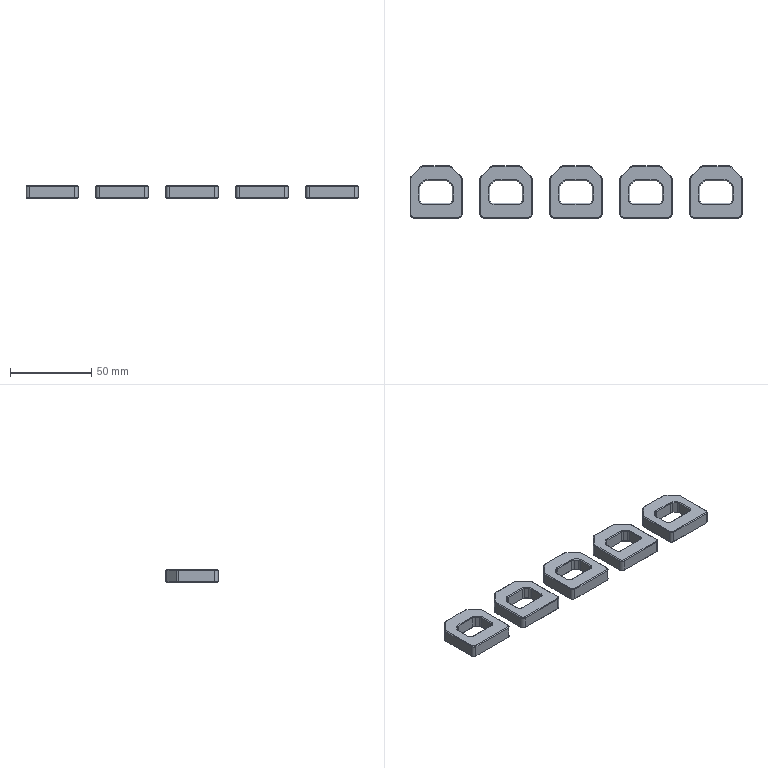NC program | NX | posted with a generic post | part box 204 x 32 x 8 mm
Lines 3530 to 3720 of 9506:
(ZLEVEL_PROFILE_COPY_1_COPY , TOOL : D10JING)
N7052 T14 M6
N7054 G54
N7056 G17 G0 G90 X47. Y0.911 S9500 M3
N7058 G43 Z30. H14
N7060 Z-7.
N7062 G94 G1 Z-8. F1000.
N7064 X47.386 Y1.134
N7066 G3 X47.886 Y2. R1.
N7068 G1 X38.071 F1200.
N7070 X38. Y1.929
N7072 Y-2.
N7074 X48.
N7076 Y1.929
N7078 X47.999 Y1.993
N7080 X47.944 Y2.027
N7082 X47.886 Y2.
N7084 G3 X47.155 Y1.318 R1.
N7086 G1 X47. Y0.811
N7088 Z-7.
N7090 G0 Z53.
N7092 X82. Y-0.845
N7094 Z-7.
N7096 G1 Z-8. F1000.
N7098 X81.5 Y-1.134
N7100 G3 X81. Y-2. R1.
N7102 G1 X91. F1200.
N7104 Y1.929
N7106 X90.919 Y2.
N7108 X81.071
N7110 X81. Y1.929
N7112 Y-2.
N7114 G3 X81.866 Y-1.5 R1.
N7116 G1 X82.155 Y-1.
N7118 Z-7.
N7120 G0 Z53.
N7122 X-4. Y-0.845
N7124 Z-7.
N7126 G1 Z-8. F1000.
N7128 X-4.5 Y-1.134
N7130 G3 X-5. Y-2. R1.
N7132 G1 X5. F1200.
N7134 Y1.929
N7136 X4.929 Y2.
N7138 X-4.929
N7140 X-5. Y1.929
N7142 Y-2.
N7144 G3 X-4.134 Y-1.5 R1.
N7146 G1 X-3.845 Y-1.
N7148 Z-7.
N7150 G0 Z53.
N7152 X-90. Y-0.845
N7154 Z-7.
N7156 G1 Z-8. F1000.
N7158 X-90.5 Y-1.134
N7160 G3 X-91. Y-2. R1.
N7162 G1 X-81. F1200.
N7164 Y1.929
N7166 X-81.071 Y2.
N7168 X-90.929
N7170 X-91. Y1.929
N7172 Y-2.
N7174 G3 X-90.134 Y-1.5 R1.
N7176 G1 X-89.845 Y-1.
N7178 Z-7.
N7180 G0 Z53.
N7182 X-39. Y0.911
N7184 Z-7.
N7186 G1 Z-8. F1000.
N7188 X-38.613 Y1.134
N7190 G3 X-38.113 Y2. R1.
N7192 G1 X-47.929 F1200.
N7194 X-48. Y1.929
N7196 Y-2.
N7198 X-38.
N7200 Y1.929
N7202 X-38.001 Y1.993
N7204 X-38.056 Y2.027
N7206 X-38.113 Y2.
N7208 G3 X-38.845 Y1.319 R1.
N7210 G1 X-39. Y0.815
N7212 Z-7.
N7214 G0 Z53.
N7216 X-27.89 Y-21.923
N7218 Z-7.
N7220 G1 Z-8. F1000.
N7222 X-28.134 Y-21.5
N7224 G3 X-29. Y-21. R1.
N7226 G1 X-57. F1200.
N7228 G2 X-64. Y-14. R7.
N7230 G1 Y8.172
N7232 G2 X-61.95 Y13.121 R7.
N7234 G1 X-56.121 Y18.95
N7236 G2 X-51.172 Y21. R7.
N7238 G1 X-34.828
N7240 G2 X-29.879 Y18.95 R7.
N7242 G1 X-24.05 Y13.121
N7244 G2 X-22. Y8.172 R7.
N7246 G1 Y-14.
N7248 G2 X-29. Y-21. R7.
N7250 G3 X-29.866 Y-21.5 R1.
N7252 G1 X-30.155 Y-22.
N7254 Z-7.
N7256 G0 Z30.
N7258 X-70.89 Y-21.923
N7260 Z-7.
N7262 G1 Z-8. F1000.
N7264 X-71.134 Y-21.5
N7266 G3 X-72. Y-21. R1.
N7268 G1 X-100. F1200.
N7270 G2 X-107. Y-14. R7.
N7272 G1 Y8.172
N7274 G2 X-104.95 Y13.121 R7.
N7276 G1 X-99.121 Y18.95
N7278 G2 X-94.172 Y21. R7.
N7280 G1 X-77.828
N7282 G2 X-72.879 Y18.95 R7.
N7284 G1 X-67.05 Y13.121
N7286 G2 X-65. Y8.172 R7.
N7288 G1 Y-14.
N7290 G2 X-72. Y-21. R7.
N7292 G3 X-72.866 Y-21.5 R1.
N7294 G1 X-73.155 Y-22.
N7296 Z-7.
N7298 G0 Z30.
N7300 X15.11 Y-21.923
N7302 Z-7.
N7304 G1 Z-8. F1000.
N7306 X14.866 Y-21.5
N7308 G3 X14. Y-21. R1.
N7310 G1 X-14. F1200.
N7312 G2 X-21. Y-14. R7.
N7314 G1 Y8.172
N7316 G2 X-18.95 Y13.121 R7.
N7318 G1 X-13.121 Y18.95
N7320 G2 X-8.172 Y21. R7.
N7322 G1 X8.172
N7324 G2 X13.121 Y18.95 R7.
N7326 G1 X18.95 Y13.121
N7328 G2 X21. Y8.172 R7.
N7330 G1 Y-14.
N7332 G2 X14. Y-21. R7.
N7334 G3 X13.134 Y-21.5 R1.
N7336 G1 X12.845 Y-22.
N7338 Z-7.
N7340 G0 Z30.
N7342 X101.11 Y-21.923
N7344 Z-7.
N7346 G1 Z-8. F1000.
N7348 X100.866 Y-21.5
N7350 G3 X100. Y-21. R1.
N7352 G1 X72. F1200.
N7354 G2 X65. Y-14. R7.
N7356 G1 Y8.172
N7358 G2 X67.05 Y13.121 R7.
N7360 G1 X72.879 Y18.95
N7362 G2 X77.828 Y21. R7.
N7364 G1 X94.172
N7366 G2 X99.121 Y18.95 R7.
N7368 G1 X104.95 Y13.121
N7370 G2 X107. Y8.172 R7.
N7372 G1 Y-14.
N7374 G2 X100. Y-21. R7.
N7376 G3 X99.134 Y-21.5 R1.
N7378 G1 X98.845 Y-22.
N7380 Z-7.
N7382 G0 Z30.
N7384 X58.11 Y-21.923
N7386 Z-7.
N7388 G1 Z-8. F1000.
N7390 X57.866 Y-21.5
N7392 G3 X57. Y-21. R1.
N7394 G1 X29. F1200.
N7396 G2 X22. Y-14. R7.
N7398 G1 Y8.172
N7400 G2 X24.05 Y13.121 R7.
N7402 G1 X29.879 Y18.95
N7404 G2 X34.828 Y21. R7.
N7406 G1 X51.172
N7408 G2 X56.121 Y18.95 R7.
N7410 G1 X61.95 Y13.121
N7412 G2 X64. Y8.172 R7.
N7414 G1 Y-14.
N7416 G2 X57. Y-21. R7.
N7418 G3 X56.134 Y-21.5 R1.
N7420 G1 X55.845 Y-22.
N7422 Z-7.
N7424 G0 Z30.
N7426 M5